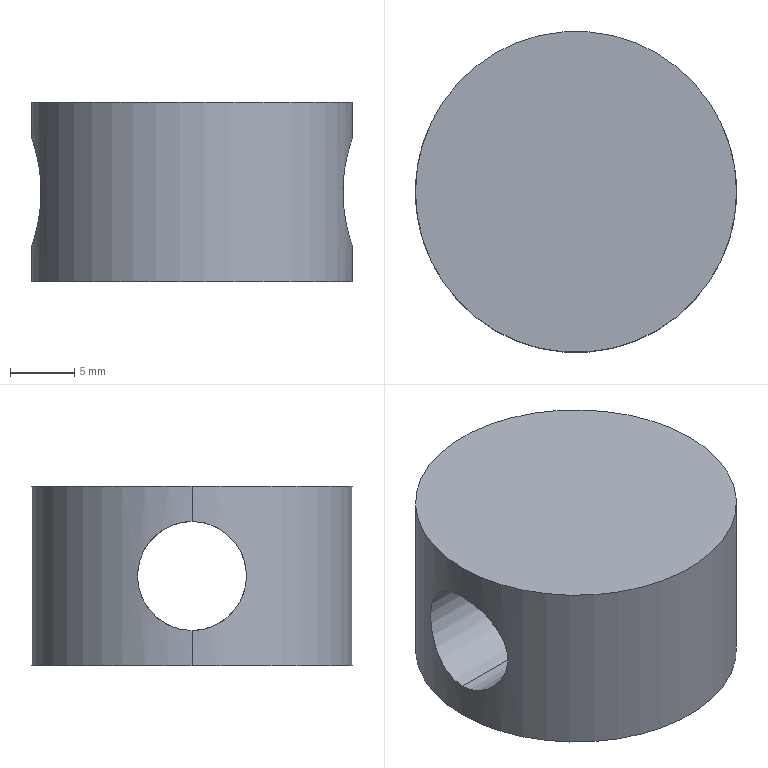Part | STEP file | Bronze shaft QY-1-15 | 1 solid | 6 faces | box 25 x 25 x 14 mm | volume 5474 mm3 | cylinder 4 | plane 2 | commonest cylinder face diameters 8.5 x2 25 x2
STEP:
#1=CARTESIAN_POINT('',(0.,0.,0.));
#2=DIRECTION('',(0.,0.,1.));
#3=DIRECTION('',(1.,0.,0.));
#4=AXIS2_PLACEMENT_3D('',#1,#2,#3);
#5=CARTESIAN_POINT('',(12.5,0.,11.25));
#6=VERTEX_POINT('',#5);
#7=CARTESIAN_POINT('',(-12.5,0.,11.25));
#8=VERTEX_POINT('',#7);
#9=CARTESIAN_POINT('',(0.,0.,11.25));
#10=DIRECTION('',(-1.,0.,0.));
#11=VECTOR('',#10,1.);
#12=LINE('',#9,#11);
#13=CARTESIAN_POINT('',(0.,0.,7.));
#14=DIRECTION('',(-1.,0.,0.));
#15=DIRECTION('',(0.,0.,1.));
#16=AXIS2_PLACEMENT_3D('',#13,#14,#15);
#17=CYLINDRICAL_SURFACE('',#16,4.25);
#18=CARTESIAN_POINT('',(6.283,0.));
#19=DIRECTION('',(0.,1.));
#20=VECTOR('',#19,1.);
#21=LINE('',#18,#20);
#22=(GEOMETRIC_REPRESENTATION_CONTEXT(2)PARAMETRIC_REPRESENTATION_CONTEXT()REPRESENTATION_CONTEXT('',''));
#23=DEFINITIONAL_REPRESENTATION('',(#21),#22);
#24=PCURVE('',#17,#23);
#25=CARTESIAN_POINT('',(0.,0.,7.));
#26=DIRECTION('',(-1.,0.,0.));
#27=DIRECTION('',(0.,0.,1.));
#28=AXIS2_PLACEMENT_3D('',#25,#26,#27);
#29=CYLINDRICAL_SURFACE('',#28,4.25);
#30=CARTESIAN_POINT('',(0.,0.));
#31=DIRECTION('',(0.,1.));
#32=VECTOR('',#31,1.);
#33=LINE('',#30,#32);
#34=(GEOMETRIC_REPRESENTATION_CONTEXT(2)PARAMETRIC_REPRESENTATION_CONTEXT()REPRESENTATION_CONTEXT('',''));
#35=DEFINITIONAL_REPRESENTATION('',(#33),#34);
#36=PCURVE('',#29,#35);
#37=SURFACE_CURVE('',#12,(#24,#36),.PCURVE_S1.);
#38=EDGE_CURVE('',#6,#8,#37,.T.);
#39=ORIENTED_EDGE('',*,*,#38,.T.);
#40=CARTESIAN_POINT('',(-12.5,0.,2.75));
#41=VERTEX_POINT('',#40);
#42=CARTESIAN_POINT('',(-12.5,0.,11.25));
#43=CARTESIAN_POINT('',(-12.5,-0.2831,11.25));
#44=CARTESIAN_POINT('',(-12.49,-0.561,11.222));
#45=CARTESIAN_POINT('',(-12.454,-1.107,11.113));
#46=CARTESIAN_POINT('',(-12.426,-1.378,11.03));
#47=CARTESIAN_POINT('',(-12.359,-1.892,10.816));
#48=CARTESIAN_POINT('',(-12.318,-2.136,10.685));
#49=CARTESIAN_POINT('',(-12.23,-2.596,10.376));
#50=CARTESIAN_POINT('',(-12.181,-2.812,10.198));
#51=CARTESIAN_POINT('',(-12.085,-3.201,9.809));
#52=CARTESIAN_POINT('',(-12.037,-3.376,9.597));
#53=CARTESIAN_POINT('',(-11.945,-3.687,9.133));
#54=CARTESIAN_POINT('',(-11.903,-3.817,8.889));
#55=CARTESIAN_POINT('',(-11.833,-4.03,8.379));
#56=CARTESIAN_POINT('',(-11.804,-4.112,8.109));
#57=CARTESIAN_POINT('',(-11.765,-4.222,7.559));
#58=CARTESIAN_POINT('',(-11.755,-4.25,7.282));
#59=CARTESIAN_POINT('',(-11.755,-4.25,6.723));
#60=CARTESIAN_POINT('',(-11.766,-4.222,6.439));
#61=CARTESIAN_POINT('',(-11.804,-4.112,5.892));
#62=CARTESIAN_POINT('',(-11.833,-4.031,5.626));
#63=CARTESIAN_POINT('',(-11.904,-3.816,5.108));
#64=CARTESIAN_POINT('',(-11.946,-3.684,4.864));
#65=CARTESIAN_POINT('',(-12.036,-3.377,4.405));
#66=CARTESIAN_POINT('',(-12.085,-3.2,4.189));
#67=CARTESIAN_POINT('',(-12.182,-2.808,3.798));
#68=CARTESIAN_POINT('',(-12.23,-2.596,3.624));
#69=CARTESIAN_POINT('',(-12.318,-2.137,3.316));
#70=CARTESIAN_POINT('',(-12.359,-1.888,3.182));
#71=CARTESIAN_POINT('',(-12.427,-1.376,2.97));
#72=CARTESIAN_POINT('',(-12.454,-1.111,2.888));
#73=CARTESIAN_POINT('',(-12.49,-0.5605,2.778));
#74=CARTESIAN_POINT('',(-12.5,-0.2789,2.75));
#75=CARTESIAN_POINT('',(-12.5,0.,2.75));
#76=B_SPLINE_CURVE_WITH_KNOTS('',3,(#42,#43,#44,#45,#46,#47,#48,#49,#50,#51,#52,#53,#54,#55,#56,#57,#58,#59,#60,#61,#62,#63,#64,#65,#66,#67,#68,#69,#70,#71,#72,#73,#74,#75),.UNSPECIFIED.,.F.,.F.,(4,2,2,2,2,2,2,2,2,2,2,2,2,2,2,2,4),(0.,0.0008368,0.001674,0.00251,0.003347,0.004184,0.005021,0.005857,0.006694,0.007531,0.008368,0.009204,0.01004,0.01088,0.01171,0.01255,0.01339),.UNSPECIFIED.);
#77=CARTESIAN_POINT('',(6.283,12.5));
#78=CARTESIAN_POINT('',(6.267,12.5));
#79=CARTESIAN_POINT('',(6.235,12.499));
#80=CARTESIAN_POINT('',(6.187,12.494));
#81=CARTESIAN_POINT('',(6.139,12.486));
#82=CARTESIAN_POINT('',(6.092,12.474));
#83=CARTESIAN_POINT('',(6.044,12.46));
#84=CARTESIAN_POINT('',(5.996,12.442));
#85=CARTESIAN_POINT('',(5.948,12.422));
#86=CARTESIAN_POINT('',(5.9,12.399));
#87=CARTESIAN_POINT('',(5.853,12.374));
#88=CARTESIAN_POINT('',(5.805,12.346));
#89=CARTESIAN_POINT('',(5.758,12.317));
#90=CARTESIAN_POINT('',(5.711,12.286));
#91=CARTESIAN_POINT('',(5.663,12.254));
#92=CARTESIAN_POINT('',(5.616,12.22));
#93=CARTESIAN_POINT('',(5.568,12.186));
#94=CARTESIAN_POINT('',(5.521,12.151));
#95=CARTESIAN_POINT('',(5.474,12.116));
#96=CARTESIAN_POINT('',(5.427,12.081));
#97=CARTESIAN_POINT('',(5.38,12.046));
#98=CARTESIAN_POINT('',(5.332,12.012));
#99=CARTESIAN_POINT('',(5.284,11.978));
#100=CARTESIAN_POINT('',(5.237,11.946));
#101=CARTESIAN_POINT('',(5.19,11.916));
#102=CARTESIAN_POINT('',(5.142,11.888));
#103=CARTESIAN_POINT('',(5.095,11.862));
#104=CARTESIAN_POINT('',(5.048,11.838));
#105=CARTESIAN_POINT('',(5.,11.816));
#106=CARTESIAN_POINT('',(4.952,11.798));
#107=CARTESIAN_POINT('',(4.904,11.783));
#108=CARTESIAN_POINT('',(4.856,11.77));
#109=CARTESIAN_POINT('',(4.808,11.762));
#110=CARTESIAN_POINT('',(4.761,11.757));
#111=CARTESIAN_POINT('',(4.713,11.755));
#112=CARTESIAN_POINT('',(4.665,11.756));
#113=CARTESIAN_POINT('',(4.617,11.762));
#114=CARTESIAN_POINT('',(4.569,11.771));
#115=CARTESIAN_POINT('',(4.521,11.783));
#116=CARTESIAN_POINT('',(4.473,11.798));
#117=CARTESIAN_POINT('',(4.425,11.816));
#118=CARTESIAN_POINT('',(4.378,11.837));
#119=CARTESIAN_POINT('',(4.33,11.861));
#120=CARTESIAN_POINT('',(4.282,11.888));
#121=CARTESIAN_POINT('',(4.234,11.916));
#122=CARTESIAN_POINT('',(4.187,11.947));
#123=CARTESIAN_POINT('',(4.14,11.979));
#124=CARTESIAN_POINT('',(4.093,12.012));
#125=CARTESIAN_POINT('',(4.045,12.046));
#126=CARTESIAN_POINT('',(3.998,12.081));
#127=CARTESIAN_POINT('',(3.95,12.116));
#128=CARTESIAN_POINT('',(3.903,12.151));
#129=CARTESIAN_POINT('',(3.856,12.186));
#130=CARTESIAN_POINT('',(3.809,12.22));
#131=CARTESIAN_POINT('',(3.762,12.254));
#132=CARTESIAN_POINT('',(3.714,12.286));
#133=CARTESIAN_POINT('',(3.667,12.317));
#134=CARTESIAN_POINT('',(3.619,12.347));
#135=CARTESIAN_POINT('',(3.571,12.374));
#136=CARTESIAN_POINT('',(3.524,12.399));
#137=CARTESIAN_POINT('',(3.477,12.422));
#138=CARTESIAN_POINT('',(3.429,12.442));
#139=CARTESIAN_POINT('',(3.382,12.46));
#140=CARTESIAN_POINT('',(3.334,12.474));
#141=CARTESIAN_POINT('',(3.285,12.486));
#142=CARTESIAN_POINT('',(3.237,12.494));
#143=CARTESIAN_POINT('',(3.189,12.499));
#144=CARTESIAN_POINT('',(3.157,12.5));
#145=CARTESIAN_POINT('',(3.142,12.5));
#146=B_SPLINE_CURVE_WITH_KNOTS('',3,(#77,#78,#79,#80,#81,#82,#83,#84,#85,#86,#87,#88,#89,#90,#91,#92,#93,#94,#95,#96,#97,#98,#99,#100,#101,#102,#103,#104,#105,#106,#107,#108,#109,#110,#111,#112,#113,#114,#115,#116,#117,#118,#119,#120,#121,#122,#123,#124,#125,#126,#127,#128,#129,#130,#131,#132,#133,#134,#135,#136,#137,#138,#139,#140,#141,#142,#143,#144,#145),.UNSPECIFIED.,.F.,.F.,(4,1,1,1,1,1,1,1,1,1,1,1,1,1,1,1,1,1,1,1,1,1,1,1,1,1,1,1,1,1,1,1,1,1,1,1,1,1,1,1,1,1,1,1,1,1,1,1,1,1,1,1,1,1,1,1,1,1,1,1,1,1,1,1,1,1,4),(0.,0.0002028,0.0004057,0.0006085,0.0008114,0.001014,0.001217,0.00142,0.001623,0.001826,0.002028,0.002231,0.002434,0.002637,0.00284,0.003043,0.003246,0.003448,0.003651,0.003854,0.004057,0.00426,0.004463,0.004666,0.004868,0.005071,0.005274,0.005477,0.00568,0.005883,0.006085,0.006288,0.006491,0.006694,0.006897,0.0071,0.007303,0.007505,0.007708,0.007911,0.008114,0.008317,0.00852,0.008722,0.008925,0.009128,0.009331,0.009534,0.009737,0.00994,0.01014,0.01035,0.01055,0.01075,0.01095,0.01116,0.01136,0.01156,0.01177,0.01197,0.01217,0.01237,0.01258,0.01278,0.01298,0.01319,0.01339),.QUASI_UNIFORM_KNOTS.);
#147=(GEOMETRIC_REPRESENTATION_CONTEXT(2)PARAMETRIC_REPRESENTATION_CONTEXT()REPRESENTATION_CONTEXT('',''));
#148=DEFINITIONAL_REPRESENTATION('',(#146),#147);
#149=PCURVE('',#17,#148);
#150=CARTESIAN_POINT('',(0.,0.,14.));
#151=DIRECTION('',(0.,0.,-1.));
#152=DIRECTION('',(-1.,0.,0.));
#153=AXIS2_PLACEMENT_3D('',#150,#151,#152);
#154=CYLINDRICAL_SURFACE('',#153,12.5);
#155=CARTESIAN_POINT('',(6.283,2.75));
#156=CARTESIAN_POINT('',(6.278,2.75));
#157=CARTESIAN_POINT('',(6.267,2.753));
#158=CARTESIAN_POINT('',(6.251,2.768));
#159=CARTESIAN_POINT('',(6.234,2.792));
#160=CARTESIAN_POINT('',(6.218,2.826));
#161=CARTESIAN_POINT('',(6.202,2.87));
#162=CARTESIAN_POINT('',(6.187,2.923));
#163=CARTESIAN_POINT('',(6.171,2.985));
#164=CARTESIAN_POINT('',(6.156,3.057));
#165=CARTESIAN_POINT('',(6.141,3.137));
#166=CARTESIAN_POINT('',(6.126,3.225));
#167=CARTESIAN_POINT('',(6.112,3.322));
#168=CARTESIAN_POINT('',(6.098,3.426));
#169=CARTESIAN_POINT('',(6.084,3.54));
#170=CARTESIAN_POINT('',(6.071,3.661));
#171=CARTESIAN_POINT('',(6.058,3.79));
#172=CARTESIAN_POINT('',(6.046,3.925));
#173=CARTESIAN_POINT('',(6.034,4.067));
#174=CARTESIAN_POINT('',(6.023,4.215));
#175=CARTESIAN_POINT('',(6.013,4.369));
#176=CARTESIAN_POINT('',(6.003,4.53));
#177=CARTESIAN_POINT('',(5.993,4.698));
#178=CARTESIAN_POINT('',(5.984,4.87));
#179=CARTESIAN_POINT('',(5.976,5.047));
#180=CARTESIAN_POINT('',(5.969,5.227));
#181=CARTESIAN_POINT('',(5.962,5.412));
#182=CARTESIAN_POINT('',(5.956,5.601));
#183=CARTESIAN_POINT('',(5.951,5.795));
#184=CARTESIAN_POINT('',(5.946,5.992));
#185=CARTESIAN_POINT('',(5.943,6.191));
#186=CARTESIAN_POINT('',(5.94,6.392));
#187=CARTESIAN_POINT('',(5.938,6.593));
#188=CARTESIAN_POINT('',(5.937,6.795));
#189=CARTESIAN_POINT('',(5.936,6.998));
#190=CARTESIAN_POINT('',(5.937,7.202));
#191=CARTESIAN_POINT('',(5.938,7.406));
#192=CARTESIAN_POINT('',(5.94,7.61));
#193=CARTESIAN_POINT('',(5.943,7.811));
#194=CARTESIAN_POINT('',(5.946,8.008));
#195=CARTESIAN_POINT('',(5.951,8.204));
#196=CARTESIAN_POINT('',(5.956,8.396));
#197=CARTESIAN_POINT('',(5.962,8.586));
#198=CARTESIAN_POINT('',(5.969,8.774));
#199=CARTESIAN_POINT('',(5.976,8.955));
#200=CARTESIAN_POINT('',(5.985,9.132));
#201=CARTESIAN_POINT('',(5.993,9.304));
#202=CARTESIAN_POINT('',(6.003,9.47));
#203=CARTESIAN_POINT('',(6.013,9.631));
#204=CARTESIAN_POINT('',(6.023,9.786));
#205=CARTESIAN_POINT('',(6.035,9.936));
#206=CARTESIAN_POINT('',(6.046,10.078));
#207=CARTESIAN_POINT('',(6.059,10.212));
#208=CARTESIAN_POINT('',(6.071,10.34));
#209=CARTESIAN_POINT('',(6.084,10.46));
#210=CARTESIAN_POINT('',(6.098,10.573));
#211=CARTESIAN_POINT('',(6.112,10.678));
#212=CARTESIAN_POINT('',(6.126,10.776));
#213=CARTESIAN_POINT('',(6.141,10.865));
#214=CARTESIAN_POINT('',(6.156,10.945));
#215=CARTESIAN_POINT('',(6.171,11.015));
#216=CARTESIAN_POINT('',(6.187,11.077));
#217=CARTESIAN_POINT('',(6.202,11.13));
#218=CARTESIAN_POINT('',(6.218,11.174));
#219=CARTESIAN_POINT('',(6.234,11.208));
#220=CARTESIAN_POINT('',(6.251,11.232));
#221=CARTESIAN_POINT('',(6.267,11.247));
#222=CARTESIAN_POINT('',(6.278,11.25));
#223=CARTESIAN_POINT('',(6.283,11.25));
#224=B_SPLINE_CURVE_WITH_KNOTS('',3,(#155,#156,#157,#158,#159,#160,#161,#162,#163,#164,#165,#166,#167,#168,#169,#170,#171,#172,#173,#174,#175,#176,#177,#178,#179,#180,#181,#182,#183,#184,#185,#186,#187,#188,#189,#190,#191,#192,#193,#194,#195,#196,#197,#198,#199,#200,#201,#202,#203,#204,#205,#206,#207,#208,#209,#210,#211,#212,#213,#214,#215,#216,#217,#218,#219,#220,#221,#222,#223),.UNSPECIFIED.,.F.,.F.,(4,1,1,1,1,1,1,1,1,1,1,1,1,1,1,1,1,1,1,1,1,1,1,1,1,1,1,1,1,1,1,1,1,1,1,1,1,1,1,1,1,1,1,1,1,1,1,1,1,1,1,1,1,1,1,1,1,1,1,1,1,1,1,1,1,1,4),(0.,0.0002028,0.0004057,0.0006085,0.0008114,0.001014,0.001217,0.00142,0.001623,0.001826,0.002028,0.002231,0.002434,0.002637,0.00284,0.003043,0.003246,0.003448,0.003651,0.003854,0.004057,0.00426,0.004463,0.004666,0.004868,0.005071,0.005274,0.005477,0.00568,0.005883,0.006085,0.006288,0.006491,0.006694,0.006897,0.0071,0.007303,0.007505,0.007708,0.007911,0.008114,0.008317,0.00852,0.008722,0.008925,0.009128,0.009331,0.009534,0.009737,0.00994,0.01014,0.01035,0.01055,0.01075,0.01095,0.01116,0.01136,0.01156,0.01177,0.01197,0.01217,0.01237,0.01258,0.01278,0.01298,0.01319,0.01339),.QUASI_UNIFORM_KNOTS.);
#225=(GEOMETRIC_REPRESENTATION_CONTEXT(2)PARAMETRIC_REPRESENTATION_CONTEXT()REPRESENTATION_CONTEXT('',''));
#226=DEFINITIONAL_REPRESENTATION('',(#224),#225);
#227=PCURVE('',#154,#226);
#228=SURFACE_CURVE('',#76,(#149,#227),.PCURVE_S1.);
#229=EDGE_CURVE('',#8,#41,#228,.T.);
#230=ORIENTED_EDGE('',*,*,#229,.T.);
#231=CARTESIAN_POINT('',(12.5,0.,2.75));
#232=VERTEX_POINT('',#231);
#233=CARTESIAN_POINT('',(0.,0.,2.75));
#234=DIRECTION('',(-1.,0.,0.));
#235=VECTOR('',#234,1.);
#236=LINE('',#233,#235);
#237=CARTESIAN_POINT('',(3.142,0.));
#238=DIRECTION('',(0.,1.));
#239=VECTOR('',#238,1.);
#240=LINE('',#237,#239);
#241=(GEOMETRIC_REPRESENTATION_CONTEXT(2)PARAMETRIC_REPRESENTATION_CONTEXT()REPRESENTATION_CONTEXT('',''));
#242=DEFINITIONAL_REPRESENTATION('',(#240),#241);
#243=PCURVE('',#17,#242);
#244=CARTESIAN_POINT('',(3.142,0.));
#245=DIRECTION('',(0.,1.));
#246=VECTOR('',#245,1.);
#247=LINE('',#244,#246);
#248=(GEOMETRIC_REPRESENTATION_CONTEXT(2)PARAMETRIC_REPRESENTATION_CONTEXT()REPRESENTATION_CONTEXT('',''));
#249=DEFINITIONAL_REPRESENTATION('',(#247),#248);
#250=PCURVE('',#29,#249);
#251=SURFACE_CURVE('',#236,(#243,#250),.PCURVE_S1.);
#252=EDGE_CURVE('',#232,#41,#251,.T.);
#253=ORIENTED_EDGE('',*,*,#252,.F.);
#254=CARTESIAN_POINT('',(12.5,0.,2.75));
#255=CARTESIAN_POINT('',(12.5,-0.2788,2.75));
#256=CARTESIAN_POINT('',(12.491,-0.5597,2.778));
#257=CARTESIAN_POINT('',(12.454,-1.111,2.888));
#258=CARTESIAN_POINT('',(12.427,-1.377,2.97));
#259=CARTESIAN_POINT('',(12.359,-1.89,3.183));
#260=CARTESIAN_POINT('',(12.318,-2.138,3.317));
#261=CARTESIAN_POINT('',(12.229,-2.597,3.624));
#262=CARTESIAN_POINT('',(12.182,-2.81,3.799));
#263=CARTESIAN_POINT('',(12.036,-3.398,4.388));
#264=CARTESIAN_POINT('',(11.939,-3.709,4.852));
#265=CARTESIAN_POINT('',(11.833,-4.031,5.626));
#266=CARTESIAN_POINT('',(11.804,-4.112,5.891));
#267=CARTESIAN_POINT('',(11.766,-4.222,6.437));
#268=CARTESIAN_POINT('',(11.755,-4.25,6.721));
#269=CARTESIAN_POINT('',(11.755,-4.25,7.281));
#270=CARTESIAN_POINT('',(11.765,-4.222,7.558));
#271=CARTESIAN_POINT('',(11.804,-4.113,8.108));
#272=CARTESIAN_POINT('',(11.833,-4.03,8.378));
#273=CARTESIAN_POINT('',(11.904,-3.817,8.89));
#274=CARTESIAN_POINT('',(11.946,-3.685,9.136));
#275=CARTESIAN_POINT('',(12.037,-3.375,9.598));
#276=CARTESIAN_POINT('',(12.085,-3.2,9.81));
#277=CARTESIAN_POINT('',(12.182,-2.811,10.2));
#278=CARTESIAN_POINT('',(12.23,-2.594,10.378));
#279=CARTESIAN_POINT('',(12.319,-2.135,10.685));
#280=CARTESIAN_POINT('',(12.359,-1.892,10.816));
#281=CARTESIAN_POINT('',(12.427,-1.378,11.03));
#282=CARTESIAN_POINT('',(12.454,-1.107,11.113));
#283=CARTESIAN_POINT('',(12.49,-0.561,11.222));
#284=CARTESIAN_POINT('',(12.5,-0.283,11.25));
#285=CARTESIAN_POINT('',(12.5,0.,11.25));
#286=B_SPLINE_CURVE_WITH_KNOTS('',3,(#254,#255,#256,#257,#258,#259,#260,#261,#262,#263,#264,#265,#266,#267,#268,#269,#270,#271,#272,#273,#274,#275,#276,#277,#278,#279,#280,#281,#282,#283,#284,#285),.UNSPECIFIED.,.F.,.F.,(4,2,2,2,2,2,2,2,2,2,2,2,2,2,2,4),(0.01339,0.01422,0.01506,0.0159,0.01673,0.01841,0.01924,0.02008,0.02092,0.02175,0.02259,0.02343,0.02426,0.0251,0.02594,0.02677),.UNSPECIFIED.);
#287=CARTESIAN_POINT('',(3.142,-12.5));
#288=CARTESIAN_POINT('',(3.157,-12.5));
#289=CARTESIAN_POINT('',(3.189,-12.499));
#290=CARTESIAN_POINT('',(3.237,-12.494));
#291=CARTESIAN_POINT('',(3.285,-12.486));
#292=CARTESIAN_POINT('',(3.333,-12.474));
#293=CARTESIAN_POINT('',(3.381,-12.46));
#294=CARTESIAN_POINT('',(3.429,-12.442));
#295=CARTESIAN_POINT('',(3.477,-12.422));
#296=CARTESIAN_POINT('',(3.524,-12.399));
#297=CARTESIAN_POINT('',(3.572,-12.374));
#298=CARTESIAN_POINT('',(3.619,-12.347));
#299=CARTESIAN_POINT('',(3.667,-12.317));
#300=CARTESIAN_POINT('',(3.715,-12.286));
#301=CARTESIAN_POINT('',(3.762,-12.254));
#302=CARTESIAN_POINT('',(3.809,-12.22));
#303=CARTESIAN_POINT('',(3.856,-12.186));
#304=CARTESIAN_POINT('',(3.903,-12.151));
#305=CARTESIAN_POINT('',(3.951,-12.115));
#306=CARTESIAN_POINT('',(3.998,-12.08));
#307=CARTESIAN_POINT('',(4.046,-12.045));
#308=CARTESIAN_POINT('',(4.093,-12.011));
#309=CARTESIAN_POINT('',(4.14,-11.978));
#310=CARTESIAN_POINT('',(4.187,-11.947));
#311=CARTESIAN_POINT('',(4.235,-11.916));
#312=CARTESIAN_POINT('',(4.282,-11.888));
#313=CARTESIAN_POINT('',(4.33,-11.861));
#314=CARTESIAN_POINT('',(4.378,-11.837));
#315=CARTESIAN_POINT('',(4.425,-11.816));
#316=CARTESIAN_POINT('',(4.473,-11.798));
#317=CARTESIAN_POINT('',(4.52,-11.783));
#318=CARTESIAN_POINT('',(4.568,-11.771));
#319=CARTESIAN_POINT('',(4.616,-11.762));
#320=CARTESIAN_POINT('',(4.665,-11.757));
#321=CARTESIAN_POINT('',(4.713,-11.755));
#322=CARTESIAN_POINT('',(4.76,-11.757));
#323=CARTESIAN_POINT('',(4.808,-11.762));
#324=CARTESIAN_POINT('',(4.856,-11.77));
#325=CARTESIAN_POINT('',(4.904,-11.782));
#326=CARTESIAN_POINT('',(4.952,-11.798));
#327=CARTESIAN_POINT('',(5.,-11.816));
#328=CARTESIAN_POINT('',(5.047,-11.838));
#329=CARTESIAN_POINT('',(5.095,-11.862));
#330=CARTESIAN_POINT('',(5.143,-11.888));
#331=CARTESIAN_POINT('',(5.19,-11.916));
#332=CARTESIAN_POINT('',(5.238,-11.947));
#333=CARTESIAN_POINT('',(5.285,-11.979));
#334=CARTESIAN_POINT('',(5.333,-12.012));
#335=CARTESIAN_POINT('',(5.38,-12.046));
#336=CARTESIAN_POINT('',(5.427,-12.081));
#337=CARTESIAN_POINT('',(5.474,-12.116));
#338=CARTESIAN_POINT('',(5.521,-12.151));
#339=CARTESIAN_POINT('',(5.569,-12.186));
#340=CARTESIAN_POINT('',(5.616,-12.221));
#341=CARTESIAN_POINT('',(5.664,-12.254));
#342=CARTESIAN_POINT('',(5.711,-12.287));
#343=CARTESIAN_POINT('',(5.758,-12.317));
#344=CARTESIAN_POINT('',(5.805,-12.347));
#345=CARTESIAN_POINT('',(5.853,-12.374));
#346=CARTESIAN_POINT('',(5.9,-12.399));
#347=CARTESIAN_POINT('',(5.948,-12.422));
#348=CARTESIAN_POINT('',(5.996,-12.442));
#349=CARTESIAN_POINT('',(6.044,-12.46));
#350=CARTESIAN_POINT('',(6.092,-12.474));
#351=CARTESIAN_POINT('',(6.139,-12.486));
#352=CARTESIAN_POINT('',(6.187,-12.494));
#353=CARTESIAN_POINT('',(6.235,-12.499));
#354=CARTESIAN_POINT('',(6.267,-12.5));
#355=CARTESIAN_POINT('',(6.283,-12.5));
#356=B_SPLINE_CURVE_WITH_KNOTS('',3,(#287,#288,#289,#290,#291,#292,#293,#294,#295,#296,#297,#298,#299,#300,#301,#302,#303,#304,#305,#306,#307,#308,#309,#310,#311,#312,#313,#314,#315,#316,#317,#318,#319,#320,#321,#322,#323,#324,#325,#326,#327,#328,#329,#330,#331,#332,#333,#334,#335,#336,#337,#338,#339,#340,#341,#342,#343,#344,#345,#346,#347,#348,#349,#350,#351,#352,#353,#354,#355),.UNSPECIFIED.,.F.,.F.,(4,1,1,1,1,1,1,1,1,1,1,1,1,1,1,1,1,1,1,1,1,1,1,1,1,1,1,1,1,1,1,1,1,1,1,1,1,1,1,1,1,1,1,1,1,1,1,1,1,1,1,1,1,1,1,1,1,1,1,1,1,1,1,1,1,1,4),(0.01339,0.01359,0.01379,0.014,0.0142,0.0144,0.0146,0.01481,0.01501,0.01521,0.01542,0.01562,0.01582,0.01602,0.01623,0.01643,0.01663,0.01684,0.01704,0.01724,0.01744,0.01765,0.01785,0.01805,0.01826,0.01846,0.01866,0.01886,0.01907,0.01927,0.01947,0.01967,0.01988,0.02008,0.02028,0.02049,0.02069,0.02089,0.02109,0.0213,0.0215,0.0217,0.02191,0.02211,0.02231,0.02251,0.02272,0.02292,0.02312,0.02333,0.02353,0.02373,0.02393,0.02414,0.02434,0.02454,0.02474,0.02495,0.02515,0.02535,0.02556,0.02576,0.02596,0.02616,0.02637,0.02657,0.02677),.QUASI_UNIFORM_KNOTS.);
#357=(GEOMETRIC_REPRESENTATION_CONTEXT(2)PARAMETRIC_REPRESENTATION_CONTEXT()REPRESENTATION_CONTEXT('',''));
#358=DEFINITIONAL_REPRESENTATION('',(#356),#357);
#359=PCURVE('',#17,#358);
#360=CARTESIAN_POINT('',(3.142,11.25));
#361=CARTESIAN_POINT('',(3.147,11.25));
#362=CARTESIAN_POINT('',(3.158,11.247));
#363=CARTESIAN_POINT('',(3.174,11.232));
#364=CARTESIAN_POINT('',(3.19,11.208));
#365=CARTESIAN_POINT('',(3.206,11.174));
#366=CARTESIAN_POINT('',(3.222,11.13));
#367=CARTESIAN_POINT('',(3.238,11.077));
#368=CARTESIAN_POINT('',(3.254,11.015));
#369=CARTESIAN_POINT('',(3.269,10.944));
#370=CARTESIAN_POINT('',(3.284,10.864));
#371=CARTESIAN_POINT('',(3.299,10.775));
#372=CARTESIAN_POINT('',(3.313,10.678));
#373=CARTESIAN_POINT('',(3.327,10.572));
#374=CARTESIAN_POINT('',(3.341,10.459));
#375=CARTESIAN_POINT('',(3.354,10.339));
#376=CARTESIAN_POINT('',(3.366,10.211));
#377=CARTESIAN_POINT('',(3.379,10.076));
#378=CARTESIAN_POINT('',(3.39,9.933));
#379=CARTESIAN_POINT('',(3.402,9.784));
#380=CARTESIAN_POINT('',(3.412,9.629));
#381=CARTESIAN_POINT('',(3.422,9.469));
#382=CARTESIAN_POINT('',(3.432,9.303));
#383=CARTESIAN_POINT('',(3.44,9.131));
#384=CARTESIAN_POINT('',(3.448,8.954));
#385=CARTESIAN_POINT('',(3.456,8.773));
#386=CARTESIAN_POINT('',(3.463,8.586));
#387=CARTESIAN_POINT('',(3.469,8.396));
#388=CARTESIAN_POINT('',(3.474,8.204));
#389=CARTESIAN_POINT('',(3.478,8.009));
#390=CARTESIAN_POINT('',(3.482,7.812));
#391=CARTESIAN_POINT('',(3.485,7.611));
#392=CARTESIAN_POINT('',(3.487,7.408));
#393=CARTESIAN_POINT('',(3.488,7.203));
#394=CARTESIAN_POINT('',(3.489,6.999));
#395=CARTESIAN_POINT('',(3.488,6.796));
#396=CARTESIAN_POINT('',(3.487,6.594));
#397=CARTESIAN_POINT('',(3.485,6.392));
#398=CARTESIAN_POINT('',(3.482,6.192));
#399=CARTESIAN_POINT('',(3.478,5.993));
#400=CARTESIAN_POINT('',(3.474,5.796));
#401=CARTESIAN_POINT('',(3.469,5.602));
#402=CARTESIAN_POINT('',(3.463,5.412));
#403=CARTESIAN_POINT('',(3.456,5.227));
#404=CARTESIAN_POINT('',(3.448,5.046));
#405=CARTESIAN_POINT('',(3.44,4.868));
#406=CARTESIAN_POINT('',(3.431,4.696));
#407=CARTESIAN_POINT('',(3.422,4.529));
#408=CARTESIAN_POINT('',(3.412,4.368));
#409=CARTESIAN_POINT('',(3.401,4.214));
#410=CARTESIAN_POINT('',(3.39,4.066));
#411=CARTESIAN_POINT('',(3.379,3.924));
#412=CARTESIAN_POINT('',(3.366,3.788));
#413=CARTESIAN_POINT('',(3.354,3.66));
#414=CARTESIAN_POINT('',(3.34,3.538));
#415=CARTESIAN_POINT('',(3.327,3.426));
#416=CARTESIAN_POINT('',(3.313,3.321));
#417=CARTESIAN_POINT('',(3.299,3.225));
#418=CARTESIAN_POINT('',(3.284,3.136));
#419=CARTESIAN_POINT('',(3.269,3.056));
#420=CARTESIAN_POINT('',(3.254,2.985));
#421=CARTESIAN_POINT('',(3.238,2.923));
#422=CARTESIAN_POINT('',(3.222,2.869));
#423=CARTESIAN_POINT('',(3.206,2.826));
#424=CARTESIAN_POINT('',(3.19,2.792));
#425=CARTESIAN_POINT('',(3.174,2.768));
#426=CARTESIAN_POINT('',(3.158,2.753));
#427=CARTESIAN_POINT('',(3.147,2.75));
#428=CARTESIAN_POINT('',(3.142,2.75));
#429=B_SPLINE_CURVE_WITH_KNOTS('',3,(#360,#361,#362,#363,#364,#365,#366,#367,#368,#369,#370,#371,#372,#373,#374,#375,#376,#377,#378,#379,#380,#381,#382,#383,#384,#385,#386,#387,#388,#389,#390,#391,#392,#393,#394,#395,#396,#397,#398,#399,#400,#401,#402,#403,#404,#405,#406,#407,#408,#409,#410,#411,#412,#413,#414,#415,#416,#417,#418,#419,#420,#421,#422,#423,#424,#425,#426,#427,#428),.UNSPECIFIED.,.F.,.F.,(4,1,1,1,1,1,1,1,1,1,1,1,1,1,1,1,1,1,1,1,1,1,1,1,1,1,1,1,1,1,1,1,1,1,1,1,1,1,1,1,1,1,1,1,1,1,1,1,1,1,1,1,1,1,1,1,1,1,1,1,1,1,1,1,1,1,4),(0.01339,0.01359,0.01379,0.014,0.0142,0.0144,0.0146,0.01481,0.01501,0.01521,0.01542,0.01562,0.01582,0.01602,0.01623,0.01643,0.01663,0.01684,0.01704,0.01724,0.01744,0.01765,0.01785,0.01805,0.01826,0.01846,0.01866,0.01886,0.01907,0.01927,0.01947,0.01967,0.01988,0.02008,0.02028,0.02049,0.02069,0.02089,0.02109,0.0213,0.0215,0.0217,0.02191,0.02211,0.02231,0.02251,0.02272,0.02292,0.02312,0.02333,0.02353,0.02373,0.02393,0.02414,0.02434,0.02454,0.02474,0.02495,0.02515,0.02535,0.02556,0.02576,0.02596,0.02616,0.02637,0.02657,0.02677),.QUASI_UNIFORM_KNOTS.);
#430=(GEOMETRIC_REPRESENTATION_CONTEXT(2)PARAMETRIC_REPRESENTATION_CONTEXT()REPRESENTATION_CONTEXT('',''));
#431=DEFINITIONAL_REPRESENTATION('',(#429),#430);
#432=PCURVE('',#154,#431);
#433=SURFACE_CURVE('',#286,(#359,#432),.PCURVE_S1.);
#434=EDGE_CURVE('',#232,#6,#433,.T.);
#435=ORIENTED_EDGE('',*,*,#434,.T.);
#436=EDGE_LOOP('',(#39,#230,#253,#435));
#437=FACE_BOUND('',#436,.F.);
#438=ADVANCED_FACE('',(#437),#17,.F.);
#439=CARTESIAN_POINT('',(12.5,0.,14.));
#440=VERTEX_POINT('',#439);
#441=CARTESIAN_POINT('',(-12.5,0.,14.));
#442=VERTEX_POINT('',#441);
#443=CARTESIAN_POINT('',(0.,0.,14.));
#444=DIRECTION('',(0.,0.,1.));
#445=DIRECTION('',(1.,0.,0.));
#446=AXIS2_PLACEMENT_3D('',#443,#444,#445);
#447=CIRCLE('',#446,12.5);
#448=CARTESIAN_POINT('',(0.,0.,14.));
#449=DIRECTION('',(0.,0.,-1.));
#450=DIRECTION('',(-1.,0.,0.));
#451=AXIS2_PLACEMENT_3D('',#448,#449,#450);
#452=CYLINDRICAL_SURFACE('',#451,12.5);
#453=CARTESIAN_POINT('',(3.142,0.));
#454=DIRECTION('',(-1.,0.));
#455=VECTOR('',#454,1.);
#456=LINE('',#453,#455);
#457=(GEOMETRIC_REPRESENTATION_CONTEXT(2)PARAMETRIC_REPRESENTATION_CONTEXT()REPRESENTATION_CONTEXT('',''));
#458=DEFINITIONAL_REPRESENTATION('',(#456),#457);
#459=PCURVE('',#452,#458);
#460=CARTESIAN_POINT('',(0.,0.,14.));
#461=DIRECTION('',(0.,0.,1.));
#462=DIRECTION('',(1.,0.,0.));
#463=AXIS2_PLACEMENT_3D('',#460,#461,#462);
#464=PLANE('',#463);
#465=CARTESIAN_POINT('',(0.,0.));
#466=DIRECTION('',(1.,0.));
#467=AXIS2_PLACEMENT_2D('',#465,#466);
#468=CIRCLE('',#467,12.5);
#469=(GEOMETRIC_REPRESENTATION_CONTEXT(2)PARAMETRIC_REPRESENTATION_CONTEXT()REPRESENTATION_CONTEXT('',''));
#470=DEFINITIONAL_REPRESENTATION('',(#468),#469);
#471=PCURVE('',#464,#470);
#472=SURFACE_CURVE('',#447,(#459,#471),.PCURVE_S1.);
#473=EDGE_CURVE('',#440,#442,#472,.T.);
#474=ORIENTED_EDGE('',*,*,#473,.F.);
#475=CARTESIAN_POINT('',(12.5,0.,14.));
#476=DIRECTION('',(0.,0.,-1.));
#477=VECTOR('',#476,1.);
#478=LINE('',#475,#477);
#479=CARTESIAN_POINT('',(3.142,0.));
#480=DIRECTION('',(0.,1.));
#481=VECTOR('',#480,1.);
#482=LINE('',#479,#481);
#483=(GEOMETRIC_REPRESENTATION_CONTEXT(2)PARAMETRIC_REPRESENTATION_CONTEXT()REPRESENTATION_CONTEXT('',''));
#484=DEFINITIONAL_REPRESENTATION('',(#482),#483);
#485=PCURVE('',#452,#484);
#486=CARTESIAN_POINT('',(3.142,0.));
#487=DIRECTION('',(0.,1.));
#488=VECTOR('',#487,1.);
#489=LINE('',#486,#488);
#490=(GEOMETRIC_REPRESENTATION_CONTEXT(2)PARAMETRIC_REPRESENTATION_CONTEXT()REPRESENTATION_CONTEXT('',''));
#491=DEFINITIONAL_REPRESENTATION('',(#489),#490);
#492=PCURVE('',#154,#491);
#493=SURFACE_CURVE('',#478,(#485,#492),.PCURVE_S1.);
#494=EDGE_CURVE('',#440,#6,#493,.T.);
#495=ORIENTED_EDGE('',*,*,#494,.T.);
#496=CARTESIAN_POINT('',(12.5,0.,11.25));
#497=CARTESIAN_POINT('',(12.5,0.2831,11.25));
#498=CARTESIAN_POINT('',(12.49,0.561,11.222));
#499=CARTESIAN_POINT('',(12.454,1.107,11.113));
#500=CARTESIAN_POINT('',(12.426,1.378,11.03));
#501=CARTESIAN_POINT('',(12.359,1.892,10.816));
#502=CARTESIAN_POINT('',(12.318,2.136,10.685));
#503=CARTESIAN_POINT('',(12.23,2.596,10.376));
#504=CARTESIAN_POINT('',(12.181,2.812,10.198));
#505=CARTESIAN_POINT('',(12.085,3.201,9.809));
#506=CARTESIAN_POINT('',(12.037,3.376,9.597));
#507=CARTESIAN_POINT('',(11.945,3.687,9.133));
#508=CARTESIAN_POINT('',(11.903,3.817,8.889));
#509=CARTESIAN_POINT('',(11.833,4.03,8.379));
#510=CARTESIAN_POINT('',(11.804,4.112,8.109));
#511=CARTESIAN_POINT('',(11.765,4.222,7.559));
#512=CARTESIAN_POINT('',(11.755,4.25,7.282));
#513=CARTESIAN_POINT('',(11.755,4.25,6.723));
#514=CARTESIAN_POINT('',(11.766,4.222,6.439));
#515=CARTESIAN_POINT('',(11.804,4.112,5.892));
#516=CARTESIAN_POINT('',(11.833,4.031,5.626));
#517=CARTESIAN_POINT('',(11.904,3.816,5.108));
#518=CARTESIAN_POINT('',(11.946,3.684,4.864));
#519=CARTESIAN_POINT('',(12.036,3.377,4.405));
#520=CARTESIAN_POINT('',(12.085,3.2,4.189));
#521=CARTESIAN_POINT('',(12.182,2.808,3.798));
#522=CARTESIAN_POINT('',(12.23,2.596,3.624));
#523=CARTESIAN_POINT('',(12.318,2.137,3.316));
#524=CARTESIAN_POINT('',(12.359,1.888,3.182));
#525=CARTESIAN_POINT('',(12.427,1.376,2.97));
#526=CARTESIAN_POINT('',(12.454,1.111,2.888));
#527=CARTESIAN_POINT('',(12.49,0.5605,2.778));
#528=CARTESIAN_POINT('',(12.5,0.2789,2.75));
#529=CARTESIAN_POINT('',(12.5,0.,2.75));
#530=B_SPLINE_CURVE_WITH_KNOTS('',3,(#496,#497,#498,#499,#500,#501,#502,#503,#504,#505,#506,#507,#508,#509,#510,#511,#512,#513,#514,#515,#516,#517,#518,#519,#520,#521,#522,#523,#524,#525,#526,#527,#528,#529),.UNSPECIFIED.,.F.,.F.,(4,2,2,2,2,2,2,2,2,2,2,2,2,2,2,2,4),(0.,0.0008368,0.001674,0.00251,0.003347,0.004184,0.005021,0.005857,0.006694,0.007531,0.008368,0.009204,0.01004,0.01088,0.01171,0.01255,0.01339),.UNSPECIFIED.);
#531=CARTESIAN_POINT('',(3.142,2.75));
#532=CARTESIAN_POINT('',(3.136,2.75));
#533=CARTESIAN_POINT('',(3.125,2.753));
#534=CARTESIAN_POINT('',(3.109,2.768));
#535=CARTESIAN_POINT('',(3.093,2.792));
#536=CARTESIAN_POINT('',(3.077,2.826));
#537=CARTESIAN_POINT('',(3.061,2.87));
#538=CARTESIAN_POINT('',(3.045,2.923));
#539=CARTESIAN_POINT('',(3.029,2.985));
#540=CARTESIAN_POINT('',(3.014,3.057));
#541=CARTESIAN_POINT('',(2.999,3.137));
#542=CARTESIAN_POINT('',(2.984,3.225));
#543=CARTESIAN_POINT('',(2.97,3.322));
#544=CARTESIAN_POINT('',(2.956,3.426));
#545=CARTESIAN_POINT('',(2.943,3.54));
#546=CARTESIAN_POINT('',(2.929,3.661));
#547=CARTESIAN_POINT('',(2.917,3.79));
#548=CARTESIAN_POINT('',(2.904,3.925));
#549=CARTESIAN_POINT('',(2.893,4.067));
#550=CARTESIAN_POINT('',(2.882,4.215));
#551=CARTESIAN_POINT('',(2.871,4.369));
#552=CARTESIAN_POINT('',(2.861,4.53));
#553=CARTESIAN_POINT('',(2.852,4.698));
#554=CARTESIAN_POINT('',(2.843,4.87));
#555=CARTESIAN_POINT('',(2.835,5.047));
#556=CARTESIAN_POINT('',(2.827,5.227));
#557=CARTESIAN_POINT('',(2.821,5.412));
#558=CARTESIAN_POINT('',(2.815,5.601));
#559=CARTESIAN_POINT('',(2.809,5.795));
#560=CARTESIAN_POINT('',(2.805,5.992));
#561=CARTESIAN_POINT('',(2.801,6.191));
#562=CARTESIAN_POINT('',(2.798,6.392));
#563=CARTESIAN_POINT('',(2.796,6.593));
#564=CARTESIAN_POINT('',(2.795,6.795));
#565=CARTESIAN_POINT('',(2.795,6.998));
#566=CARTESIAN_POINT('',(2.795,7.202));
#567=CARTESIAN_POINT('',(2.796,7.406));
#568=CARTESIAN_POINT('',(2.798,7.61));
#569=CARTESIAN_POINT('',(2.801,7.811));
#570=CARTESIAN_POINT('',(2.805,8.008));
#571=CARTESIAN_POINT('',(2.809,8.204));
#572=CARTESIAN_POINT('',(2.815,8.396));
#573=CARTESIAN_POINT('',(2.821,8.586));
#574=CARTESIAN_POINT('',(2.827,8.774));
#575=CARTESIAN_POINT('',(2.835,8.955));
#576=CARTESIAN_POINT('',(2.843,9.132));
#577=CARTESIAN_POINT('',(2.852,9.304));
#578=CARTESIAN_POINT('',(2.861,9.47));
#579=CARTESIAN_POINT('',(2.871,9.631));
#580=CARTESIAN_POINT('',(2.882,9.786));
#581=CARTESIAN_POINT('',(2.893,9.936));
#582=CARTESIAN_POINT('',(2.905,10.078));
#583=CARTESIAN_POINT('',(2.917,10.212));
#584=CARTESIAN_POINT('',(2.93,10.34));
#585=CARTESIAN_POINT('',(2.943,10.46));
#586=CARTESIAN_POINT('',(2.956,10.573));
#587=CARTESIAN_POINT('',(2.97,10.678));
#588=CARTESIAN_POINT('',(2.985,10.776));
#589=CARTESIAN_POINT('',(2.999,10.865));
#590=CARTESIAN_POINT('',(3.014,10.945));
#591=CARTESIAN_POINT('',(3.03,11.015));
#592=CARTESIAN_POINT('',(3.045,11.077));
#593=CARTESIAN_POINT('',(3.061,11.13));
#594=CARTESIAN_POINT('',(3.077,11.174));
#595=CARTESIAN_POINT('',(3.093,11.208));
#596=CARTESIAN_POINT('',(3.109,11.232));
#597=CARTESIAN_POINT('',(3.125,11.247));
#598=CARTESIAN_POINT('',(3.136,11.25));
#599=CARTESIAN_POINT('',(3.142,11.25));
#600=B_SPLINE_CURVE_WITH_KNOTS('',3,(#531,#532,#533,#534,#535,#536,#537,#538,#539,#540,#541,#542,#543,#544,#545,#546,#547,#548,#549,#550,#551,#552,#553,#554,#555,#556,#557,#558,#559,#560,#561,#562,#563,#564,#565,#566,#567,#568,#569,#570,#571,#572,#573,#574,#575,#576,#577,#578,#579,#580,#581,#582,#583,#584,#585,#586,#587,#588,#589,#590,#591,#592,#593,#594,#595,#596,#597,#598,#599),.UNSPECIFIED.,.F.,.F.,(4,1,1,1,1,1,1,1,1,1,1,1,1,1,1,1,1,1,1,1,1,1,1,1,1,1,1,1,1,1,1,1,1,1,1,1,1,1,1,1,1,1,1,1,1,1,1,1,1,1,1,1,1,1,1,1,1,1,1,1,1,1,1,1,1,1,4),(0.,0.0002028,0.0004057,0.0006085,0.0008114,0.001014,0.001217,0.00142,0.001623,0.001826,0.002028,0.002231,0.002434,0.002637,0.00284,0.003043,0.003246,0.003448,0.003651,0.003854,0.004057,0.00426,0.004463,0.004666,0.004868,0.005071,0.005274,0.005477,0.00568,0.005883,0.006085,0.006288,0.006491,0.006694,0.006897,0.0071,0.007303,0.007505,0.007708,0.007911,0.008114,0.008317,0.00852,0.008722,0.008925,0.009128,0.009331,0.009534,0.009737,0.00994,0.01014,0.01035,0.01055,0.01075,0.01095,0.01116,0.01136,0.01156,0.01177,0.01197,0.01217,0.01237,0.01258,0.01278,0.01298,0.01319,0.01339),.QUASI_UNIFORM_KNOTS.);
#601=(GEOMETRIC_REPRESENTATION_CONTEXT(2)PARAMETRIC_REPRESENTATION_CONTEXT()REPRESENTATION_CONTEXT('',''));
#602=DEFINITIONAL_REPRESENTATION('',(#600),#601);
#603=PCURVE('',#452,#602);
#604=CARTESIAN_POINT('',(0.,-12.5));
#605=CARTESIAN_POINT('',(0.01615,-12.5));
#606=CARTESIAN_POINT('',(0.0483,-12.499));
#607=CARTESIAN_POINT('',(0.09622,-12.494));
#608=CARTESIAN_POINT('',(0.1439,-12.486));
#609=CARTESIAN_POINT('',(0.1916,-12.474));
#610=CARTESIAN_POINT('',(0.2393,-12.46));
#611=CARTESIAN_POINT('',(0.2873,-12.442));
#612=CARTESIAN_POINT('',(0.3352,-12.422));
#613=CARTESIAN_POINT('',(0.3831,-12.399));
#614=CARTESIAN_POINT('',(0.4306,-12.374));
#615=CARTESIAN_POINT('',(0.478,-12.346));
#616=CARTESIAN_POINT('',(0.5253,-12.317));
#617=CARTESIAN_POINT('',(0.5726,-12.286));
#618=CARTESIAN_POINT('',(0.62,-12.254));
#619=CARTESIAN_POINT('',(0.6675,-12.22));
#620=CARTESIAN_POINT('',(0.715,-12.186));
#621=CARTESIAN_POINT('',(0.7623,-12.151));
#622=CARTESIAN_POINT('',(0.8094,-12.116));
#623=CARTESIAN_POINT('',(0.8564,-12.081));
#624=CARTESIAN_POINT('',(0.9036,-12.046));
#625=CARTESIAN_POINT('',(0.9509,-12.012));
#626=CARTESIAN_POINT('',(0.9987,-11.978));
#627=CARTESIAN_POINT('',(1.046,-11.946));
#628=CARTESIAN_POINT('',(1.094,-11.916));
#629=CARTESIAN_POINT('',(1.141,-11.888));
#630=CARTESIAN_POINT('',(1.188,-11.862));
#631=CARTESIAN_POINT('',(1.236,-11.838));
#632=CARTESIAN_POINT('',(1.283,-11.816));
#633=CARTESIAN_POINT('',(1.331,-11.798));
#634=CARTESIAN_POINT('',(1.379,-11.783));
#635=CARTESIAN_POINT('',(1.427,-11.77));
#636=CARTESIAN_POINT('',(1.475,-11.762));
#637=CARTESIAN_POINT('',(1.523,-11.757));
#638=CARTESIAN_POINT('',(1.57,-11.755));
#639=CARTESIAN_POINT('',(1.618,-11.756));
#640=CARTESIAN_POINT('',(1.666,-11.762));
#641=CARTESIAN_POINT('',(1.715,-11.771));
#642=CARTESIAN_POINT('',(1.763,-11.783));
#643=CARTESIAN_POINT('',(1.81,-11.798));
#644=CARTESIAN_POINT('',(1.858,-11.816));
#645=CARTESIAN_POINT('',(1.905,-11.837));
#646=CARTESIAN_POINT('',(1.953,-11.861));
#647=CARTESIAN_POINT('',(2.001,-11.888));
#648=CARTESIAN_POINT('',(2.049,-11.916));
#649=CARTESIAN_POINT('',(2.096,-11.947));
#650=CARTESIAN_POINT('',(2.143,-11.979));
#651=CARTESIAN_POINT('',(2.191,-12.012));
#652=CARTESIAN_POINT('',(2.238,-12.046));
#653=CARTESIAN_POINT('',(2.285,-12.081));
#654=CARTESIAN_POINT('',(2.333,-12.116));
#655=CARTESIAN_POINT('',(2.38,-12.151));
#656=CARTESIAN_POINT('',(2.427,-12.186));
#657=CARTESIAN_POINT('',(2.474,-12.22));
#658=CARTESIAN_POINT('',(2.521,-12.254));
#659=CARTESIAN_POINT('',(2.569,-12.286));
#660=CARTESIAN_POINT('',(2.616,-12.317));
#661=CARTESIAN_POINT('',(2.664,-12.347));
#662=CARTESIAN_POINT('',(2.712,-12.374));
#663=CARTESIAN_POINT('',(2.759,-12.399));
#664=CARTESIAN_POINT('',(2.807,-12.422));
#665=CARTESIAN_POINT('',(2.854,-12.442));
#666=CARTESIAN_POINT('',(2.902,-12.46));
#667=CARTESIAN_POINT('',(2.95,-12.474));
#668=CARTESIAN_POINT('',(2.998,-12.486));
#669=CARTESIAN_POINT('',(3.046,-12.494));
#670=CARTESIAN_POINT('',(3.094,-12.499));
#671=CARTESIAN_POINT('',(3.126,-12.5));
#672=CARTESIAN_POINT('',(3.142,-12.5));
#673=B_SPLINE_CURVE_WITH_KNOTS('',3,(#604,#605,#606,#607,#608,#609,#610,#611,#612,#613,#614,#615,#616,#617,#618,#619,#620,#621,#622,#623,#624,#625,#626,#627,#628,#629,#630,#631,#632,#633,#634,#635,#636,#637,#638,#639,#640,#641,#642,#643,#644,#645,#646,#647,#648,#649,#650,#651,#652,#653,#654,#655,#656,#657,#658,#659,#660,#661,#662,#663,#664,#665,#666,#667,#668,#669,#670,#671,#672),.UNSPECIFIED.,.F.,.F.,(4,1,1,1,1,1,1,1,1,1,1,1,1,1,1,1,1,1,1,1,1,1,1,1,1,1,1,1,1,1,1,1,1,1,1,1,1,1,1,1,1,1,1,1,1,1,1,1,1,1,1,1,1,1,1,1,1,1,1,1,1,1,1,1,1,1,4),(0.,0.0002028,0.0004057,0.0006085,0.0008114,0.001014,0.001217,0.00142,0.001623,0.001826,0.002028,0.002231,0.002434,0.002637,0.00284,0.003043,0.003246,0.003448,0.003651,0.003854,0.004057,0.00426,0.004463,0.004666,0.004868,0.005071,0.005274,0.005477,0.00568,0.005883,0.006085,0.006288,0.006491,0.006694,0.006897,0.0071,0.007303,0.007505,0.007708,0.007911,0.008114,0.008317,0.00852,0.008722,0.008925,0.009128,0.009331,0.009534,0.009737,0.00994,0.01014,0.01035,0.01055,0.01075,0.01095,0.01116,0.01136,0.01156,0.01177,0.01197,0.01217,0.01237,0.01258,0.01278,0.01298,0.01319,0.01339),.QUASI_UNIFORM_KNOTS.);
#674=(GEOMETRIC_REPRESENTATION_CONTEXT(2)PARAMETRIC_REPRESENTATION_CONTEXT()REPRESENTATION_CONTEXT('',''));
#675=DEFINITIONAL_REPRESENTATION('',(#673),#674);
#676=PCURVE('',#29,#675);
#677=SURFACE_CURVE('',#530,(#603,#676),.PCURVE_S1.);
#678=EDGE_CURVE('',#6,#232,#677,.T.);
#679=ORIENTED_EDGE('',*,*,#678,.T.);
#680=CARTESIAN_POINT('',(12.5,0.,0.));
#681=VERTEX_POINT('',#680);
#682=CARTESIAN_POINT('',(12.5,0.,14.));
#683=DIRECTION('',(0.,0.,-1.));
#684=VECTOR('',#683,1.);
#685=LINE('',#682,#684);
#686=CARTESIAN_POINT('',(3.142,0.));
#687=DIRECTION('',(0.,1.));
#688=VECTOR('',#687,1.);
#689=LINE('',#686,#688);
#690=(GEOMETRIC_REPRESENTATION_CONTEXT(2)PARAMETRIC_REPRESENTATION_CONTEXT()REPRESENTATION_CONTEXT('',''));
#691=DEFINITIONAL_REPRESENTATION('',(#689),#690);
#692=PCURVE('',#452,#691);
#693=CARTESIAN_POINT('',(3.142,0.));
#694=DIRECTION('',(0.,1.));
#695=VECTOR('',#694,1.);
#696=LINE('',#693,#695);
#697=(GEOMETRIC_REPRESENTATION_CONTEXT(2)PARAMETRIC_REPRESENTATION_CONTEXT()REPRESENTATION_CONTEXT('',''));
#698=DEFINITIONAL_REPRESENTATION('',(#696),#697);
#699=PCURVE('',#154,#698);
#700=SURFACE_CURVE('',#685,(#692,#699),.PCURVE_S1.);
#701=EDGE_CURVE('',#232,#681,#700,.T.);
#702=ORIENTED_EDGE('',*,*,#701,.T.);
#703=CARTESIAN_POINT('',(-12.5,0.,0.));
#704=VERTEX_POINT('',#703);
#705=CARTESIAN_POINT('',(0.,0.,0.));
#706=DIRECTION('',(0.,0.,1.));
#707=DIRECTION('',(1.,0.,0.));
#708=AXIS2_PLACEMENT_3D('',#705,#706,#707);
#709=CIRCLE('',#708,12.5);
#710=CARTESIAN_POINT('',(3.142,14.));
#711=DIRECTION('',(-1.,0.));
#712=VECTOR('',#711,1.);
#713=LINE('',#710,#712);
#714=(GEOMETRIC_REPRESENTATION_CONTEXT(2)PARAMETRIC_REPRESENTATION_CONTEXT()REPRESENTATION_CONTEXT('',''));
#715=DEFINITIONAL_REPRESENTATION('',(#713),#714);
#716=PCURVE('',#452,#715);
#717=CARTESIAN_POINT('',(0.,0.,0.));
#718=DIRECTION('',(0.,0.,1.));
#719=DIRECTION('',(1.,0.,0.));
#720=AXIS2_PLACEMENT_3D('',#717,#718,#719);
#721=PLANE('',#720);
#722=CARTESIAN_POINT('',(0.,0.));
#723=DIRECTION('',(1.,0.));
#724=AXIS2_PLACEMENT_2D('',#722,#723);
#725=CIRCLE('',#724,12.5);
#726=(GEOMETRIC_REPRESENTATION_CONTEXT(2)PARAMETRIC_REPRESENTATION_CONTEXT()REPRESENTATION_CONTEXT('',''));
#727=DEFINITIONAL_REPRESENTATION('',(#725),#726);
#728=PCURVE('',#721,#727);
#729=SURFACE_CURVE('',#709,(#716,#728),.PCURVE_S1.);
#730=EDGE_CURVE('',#681,#704,#729,.T.);
#731=ORIENTED_EDGE('',*,*,#730,.T.);
#732=CARTESIAN_POINT('',(-12.5,0.,14.));
#733=DIRECTION('',(0.,0.,-1.));
#734=VECTOR('',#733,1.);
#735=LINE('',#732,#734);
#736=CARTESIAN_POINT('',(0.,0.));
#737=DIRECTION('',(0.,1.));
#738=VECTOR('',#737,1.);
#739=LINE('',#736,#738);
#740=(GEOMETRIC_REPRESENTATION_CONTEXT(2)PARAMETRIC_REPRESENTATION_CONTEXT()REPRESENTATION_CONTEXT('',''));
#741=DEFINITIONAL_REPRESENTATION('',(#739),#740);
#742=PCURVE('',#452,#741);
#743=CARTESIAN_POINT('',(6.283,0.));
#744=DIRECTION('',(0.,1.));
#745=VECTOR('',#744,1.);
#746=LINE('',#743,#745);
#747=(GEOMETRIC_REPRESENTATION_CONTEXT(2)PARAMETRIC_REPRESENTATION_CONTEXT()REPRESENTATION_CONTEXT('',''));
#748=DEFINITIONAL_REPRESENTATION('',(#746),#747);
#749=PCURVE('',#154,#748);
#750=SURFACE_CURVE('',#735,(#742,#749),.PCURVE_S1.);
#751=EDGE_CURVE('',#41,#704,#750,.T.);
#752=ORIENTED_EDGE('',*,*,#751,.F.);
#753=CARTESIAN_POINT('',(-12.5,0.,2.75));
#754=CARTESIAN_POINT('',(-12.5,0.2788,2.75));
#755=CARTESIAN_POINT('',(-12.491,0.5597,2.778));
#756=CARTESIAN_POINT('',(-12.454,1.111,2.888));
#757=CARTESIAN_POINT('',(-12.427,1.377,2.97));
#758=CARTESIAN_POINT('',(-12.359,1.89,3.183));
#759=CARTESIAN_POINT('',(-12.318,2.138,3.317));
#760=CARTESIAN_POINT('',(-12.229,2.597,3.624));
#761=CARTESIAN_POINT('',(-12.182,2.81,3.799));
#762=CARTESIAN_POINT('',(-12.036,3.398,4.388));
#763=CARTESIAN_POINT('',(-11.939,3.709,4.852));
#764=CARTESIAN_POINT('',(-11.833,4.031,5.626));
#765=CARTESIAN_POINT('',(-11.804,4.112,5.891));
#766=CARTESIAN_POINT('',(-11.766,4.222,6.437));
#767=CARTESIAN_POINT('',(-11.755,4.25,6.721));
#768=CARTESIAN_POINT('',(-11.755,4.25,7.281));
#769=CARTESIAN_POINT('',(-11.765,4.222,7.558));
#770=CARTESIAN_POINT('',(-11.804,4.113,8.108));
#771=CARTESIAN_POINT('',(-11.833,4.03,8.378));
#772=CARTESIAN_POINT('',(-11.904,3.817,8.89));
#773=CARTESIAN_POINT('',(-11.946,3.685,9.136));
#774=CARTESIAN_POINT('',(-12.037,3.375,9.598));
#775=CARTESIAN_POINT('',(-12.085,3.2,9.81));
#776=CARTESIAN_POINT('',(-12.182,2.811,10.2));
#777=CARTESIAN_POINT('',(-12.23,2.594,10.378));
#778=CARTESIAN_POINT('',(-12.319,2.135,10.685));
#779=CARTESIAN_POINT('',(-12.359,1.892,10.816));
#780=CARTESIAN_POINT('',(-12.427,1.378,11.03));
#781=CARTESIAN_POINT('',(-12.454,1.107,11.113));
#782=CARTESIAN_POINT('',(-12.49,0.561,11.222));
#783=CARTESIAN_POINT('',(-12.5,0.283,11.25));
#784=CARTESIAN_POINT('',(-12.5,0.,11.25));
#785=B_SPLINE_CURVE_WITH_KNOTS('',3,(#753,#754,#755,#756,#757,#758,#759,#760,#761,#762,#763,#764,#765,#766,#767,#768,#769,#770,#771,#772,#773,#774,#775,#776,#777,#778,#779,#780,#781,#782,#783,#784),.UNSPECIFIED.,.F.,.F.,(4,2,2,2,2,2,2,2,2,2,2,2,2,2,2,4),(0.01339,0.01422,0.01506,0.0159,0.01673,0.01841,0.01924,0.02008,0.02092,0.02175,0.02259,0.02343,0.02426,0.0251,0.02594,0.02677),.UNSPECIFIED.);
#786=CARTESIAN_POINT('',(0.,11.25));
#787=CARTESIAN_POINT('',(0.005407,11.25));
#788=CARTESIAN_POINT('',(0.01624,11.247));
#789=CARTESIAN_POINT('',(0.03251,11.232));
#790=CARTESIAN_POINT('',(0.04874,11.208));
#791=CARTESIAN_POINT('',(0.0649,11.174));
#792=CARTESIAN_POINT('',(0.08089,11.13));
#793=CARTESIAN_POINT('',(0.09661,11.077));
#794=CARTESIAN_POINT('',(0.1121,11.015));
#795=CARTESIAN_POINT('',(0.1273,10.944));
#796=CARTESIAN_POINT('',(0.1423,10.864));
#797=CARTESIAN_POINT('',(0.1571,10.775));
#798=CARTESIAN_POINT('',(0.1715,10.678));
#799=CARTESIAN_POINT('',(0.1855,10.572));
#800=CARTESIAN_POINT('',(0.199,10.459));
#801=CARTESIAN_POINT('',(0.2121,10.339));
#802=CARTESIAN_POINT('',(0.2248,10.211));
#803=CARTESIAN_POINT('',(0.237,10.076));
#804=CARTESIAN_POINT('',(0.2488,9.933));
#805=CARTESIAN_POINT('',(0.26,9.784));
#806=CARTESIAN_POINT('',(0.2706,9.629));
#807=CARTESIAN_POINT('',(0.2806,9.469));
#808=CARTESIAN_POINT('',(0.29,9.303));
#809=CARTESIAN_POINT('',(0.2988,9.131));
#810=CARTESIAN_POINT('',(0.3069,8.954));
#811=CARTESIAN_POINT('',(0.3143,8.773));
#812=CARTESIAN_POINT('',(0.3211,8.586));
#813=CARTESIAN_POINT('',(0.3271,8.396));
#814=CARTESIAN_POINT('',(0.3323,8.204));
#815=CARTESIAN_POINT('',(0.3367,8.009));
#816=CARTESIAN_POINT('',(0.3404,7.812));
#817=CARTESIAN_POINT('',(0.3433,7.611));
#818=CARTESIAN_POINT('',(0.3454,7.408));
#819=CARTESIAN_POINT('',(0.3466,7.203));
#820=CARTESIAN_POINT('',(0.3471,6.999));
#821=CARTESIAN_POINT('',(0.3466,6.796));
#822=CARTESIAN_POINT('',(0.3454,6.594));
#823=CARTESIAN_POINT('',(0.3433,6.392));
#824=CARTESIAN_POINT('',(0.3405,6.192));
#825=CARTESIAN_POINT('',(0.3368,5.993));
#826=CARTESIAN_POINT('',(0.3323,5.796));
#827=CARTESIAN_POINT('',(0.327,5.602));
#828=CARTESIAN_POINT('',(0.321,5.412));
#829=CARTESIAN_POINT('',(0.3143,5.227));
#830=CARTESIAN_POINT('',(0.3068,5.046));
#831=CARTESIAN_POINT('',(0.2987,4.868));
#832=CARTESIAN_POINT('',(0.2899,4.696));
#833=CARTESIAN_POINT('',(0.2804,4.529));
#834=CARTESIAN_POINT('',(0.2704,4.368));
#835=CARTESIAN_POINT('',(0.2598,4.214));
#836=CARTESIAN_POINT('',(0.2487,4.066));
#837=CARTESIAN_POINT('',(0.237,3.924));
#838=CARTESIAN_POINT('',(0.2247,3.788));
#839=CARTESIAN_POINT('',(0.212,3.66));
#840=CARTESIAN_POINT('',(0.1988,3.538));
#841=CARTESIAN_POINT('',(0.1852,3.426));
#842=CARTESIAN_POINT('',(0.1713,3.321));
#843=CARTESIAN_POINT('',(0.157,3.225));
#844=CARTESIAN_POINT('',(0.1424,3.136));
#845=CARTESIAN_POINT('',(0.1274,3.056));
#846=CARTESIAN_POINT('',(0.1121,2.985));
#847=CARTESIAN_POINT('',(0.09647,2.923));
#848=CARTESIAN_POINT('',(0.08067,2.869));
#849=CARTESIAN_POINT('',(0.06478,2.826));
#850=CARTESIAN_POINT('',(0.0488,2.792));
#851=CARTESIAN_POINT('',(0.03268,2.768));
#852=CARTESIAN_POINT('',(0.01642,2.753));
#853=CARTESIAN_POINT('',(0.005489,2.75));
#854=CARTESIAN_POINT('',(0.,2.75));
#855=B_SPLINE_CURVE_WITH_KNOTS('',3,(#786,#787,#788,#789,#790,#791,#792,#793,#794,#795,#796,#797,#798,#799,#800,#801,#802,#803,#804,#805,#806,#807,#808,#809,#810,#811,#812,#813,#814,#815,#816,#817,#818,#819,#820,#821,#822,#823,#824,#825,#826,#827,#828,#829,#830,#831,#832,#833,#834,#835,#836,#837,#838,#839,#840,#841,#842,#843,#844,#845,#846,#847,#848,#849,#850,#851,#852,#853,#854),.UNSPECIFIED.,.F.,.F.,(4,1,1,1,1,1,1,1,1,1,1,1,1,1,1,1,1,1,1,1,1,1,1,1,1,1,1,1,1,1,1,1,1,1,1,1,1,1,1,1,1,1,1,1,1,1,1,1,1,1,1,1,1,1,1,1,1,1,1,1,1,1,1,1,1,1,4),(0.01339,0.01359,0.01379,0.014,0.0142,0.0144,0.0146,0.01481,0.01501,0.01521,0.01542,0.01562,0.01582,0.01602,0.01623,0.01643,0.01663,0.01684,0.01704,0.01724,0.01744,0.01765,0.01785,0.01805,0.01826,0.01846,0.01866,0.01886,0.01907,0.01927,0.01947,0.01967,0.01988,0.02008,0.02028,0.02049,0.02069,0.02089,0.02109,0.0213,0.0215,0.0217,0.02191,0.02211,0.02231,0.02251,0.02272,0.02292,0.02312,0.02333,0.02353,0.02373,0.02393,0.02414,0.02434,0.02454,0.02474,0.02495,0.02515,0.02535,0.02556,0.02576,0.02596,0.02616,0.02637,0.02657,0.02677),.QUASI_UNIFORM_KNOTS.);
#856=(GEOMETRIC_REPRESENTATION_CONTEXT(2)PARAMETRIC_REPRESENTATION_CONTEXT()REPRESENTATION_CONTEXT('',''));
#857=DEFINITIONAL_REPRESENTATION('',(#855),#856);
#858=PCURVE('',#452,#857);
#859=CARTESIAN_POINT('',(3.142,12.5));
#860=CARTESIAN_POINT('',(3.126,12.5));
#861=CARTESIAN_POINT('',(3.094,12.499));
#862=CARTESIAN_POINT('',(3.046,12.494));
#863=CARTESIAN_POINT('',(2.998,12.486));
#864=CARTESIAN_POINT('',(2.95,12.474));
#865=CARTESIAN_POINT('',(2.902,12.46));
#866=CARTESIAN_POINT('',(2.854,12.442));
#867=CARTESIAN_POINT('',(2.807,12.422));
#868=CARTESIAN_POINT('',(2.759,12.399));
#869=CARTESIAN_POINT('',(2.711,12.374));
#870=CARTESIAN_POINT('',(2.664,12.347));
#871=CARTESIAN_POINT('',(2.616,12.317));
#872=CARTESIAN_POINT('',(2.568,12.286));
#873=CARTESIAN_POINT('',(2.521,12.254));
#874=CARTESIAN_POINT('',(2.474,12.22));
#875=CARTESIAN_POINT('',(2.427,12.186));
#876=CARTESIAN_POINT('',(2.38,12.151));
#877=CARTESIAN_POINT('',(2.332,12.115));
#878=CARTESIAN_POINT('',(2.285,12.08));
#879=CARTESIAN_POINT('',(2.238,12.045));
#880=CARTESIAN_POINT('',(2.19,12.011));
#881=CARTESIAN_POINT('',(2.143,11.978));
#882=CARTESIAN_POINT('',(2.096,11.947));
#883=CARTESIAN_POINT('',(2.048,11.916));
#884=CARTESIAN_POINT('',(2.001,11.888));
#885=CARTESIAN_POINT('',(1.953,11.861));
#886=CARTESIAN_POINT('',(1.905,11.837));
#887=CARTESIAN_POINT('',(1.858,11.816));
#888=CARTESIAN_POINT('',(1.81,11.798));
#889=CARTESIAN_POINT('',(1.763,11.783));
#890=CARTESIAN_POINT('',(1.715,11.771));
#891=CARTESIAN_POINT('',(1.667,11.762));
#892=CARTESIAN_POINT('',(1.619,11.757));
#893=CARTESIAN_POINT('',(1.571,11.755));
#894=CARTESIAN_POINT('',(1.523,11.757));
#895=CARTESIAN_POINT('',(1.475,11.762));
#896=CARTESIAN_POINT('',(1.427,11.77));
#897=CARTESIAN_POINT('',(1.38,11.782));
#898=CARTESIAN_POINT('',(1.332,11.798));
#899=CARTESIAN_POINT('',(1.284,11.816));
#900=CARTESIAN_POINT('',(1.236,11.838));
#901=CARTESIAN_POINT('',(1.188,11.862));
#902=CARTESIAN_POINT('',(1.141,11.888));
#903=CARTESIAN_POINT('',(1.093,11.916));
#904=CARTESIAN_POINT('',(1.046,11.947));
#905=CARTESIAN_POINT('',(0.998,11.979));
#906=CARTESIAN_POINT('',(0.9505,12.012));
#907=CARTESIAN_POINT('',(0.9032,12.046));
#908=CARTESIAN_POINT('',(0.8561,12.081));
#909=CARTESIAN_POINT('',(0.8091,12.116));
#910=CARTESIAN_POINT('',(0.762,12.151));
#911=CARTESIAN_POINT('',(0.7145,12.186));
#912=CARTESIAN_POINT('',(0.667,12.221));
#913=CARTESIAN_POINT('',(0.6195,12.254));
#914=CARTESIAN_POINT('',(0.5722,12.287));
#915=CARTESIAN_POINT('',(0.525,12.317));
#916=CARTESIAN_POINT('',(0.4778,12.347));
#917=CARTESIAN_POINT('',(0.4305,12.374));
#918=CARTESIAN_POINT('',(0.3829,12.399));
#919=CARTESIAN_POINT('',(0.3351,12.422));
#920=CARTESIAN_POINT('',(0.2871,12.442));
#921=CARTESIAN_POINT('',(0.2392,12.46));
#922=CARTESIAN_POINT('',(0.1915,12.474));
#923=CARTESIAN_POINT('',(0.1439,12.486));
#924=CARTESIAN_POINT('',(0.0962,12.494));
#925=CARTESIAN_POINT('',(0.04829,12.499));
#926=CARTESIAN_POINT('',(0.01614,12.5));
#927=CARTESIAN_POINT('',(0.,12.5));
#928=B_SPLINE_CURVE_WITH_KNOTS('',3,(#859,#860,#861,#862,#863,#864,#865,#866,#867,#868,#869,#870,#871,#872,#873,#874,#875,#876,#877,#878,#879,#880,#881,#882,#883,#884,#885,#886,#887,#888,#889,#890,#891,#892,#893,#894,#895,#896,#897,#898,#899,#900,#901,#902,#903,#904,#905,#906,#907,#908,#909,#910,#911,#912,#913,#914,#915,#916,#917,#918,#919,#920,#921,#922,#923,#924,#925,#926,#927),.UNSPECIFIED.,.F.,.F.,(4,1,1,1,1,1,1,1,1,1,1,1,1,1,1,1,1,1,1,1,1,1,1,1,1,1,1,1,1,1,1,1,1,1,1,1,1,1,1,1,1,1,1,1,1,1,1,1,1,1,1,1,1,1,1,1,1,1,1,1,1,1,1,1,1,1,4),(0.01339,0.01359,0.01379,0.014,0.0142,0.0144,0.0146,0.01481,0.01501,0.01521,0.01542,0.01562,0.01582,0.01602,0.01623,0.01643,0.01663,0.01684,0.01704,0.01724,0.01744,0.01765,0.01785,0.01805,0.01826,0.01846,0.01866,0.01886,0.01907,0.01927,0.01947,0.01967,0.01988,0.02008,0.02028,0.02049,0.02069,0.02089,0.02109,0.0213,0.0215,0.0217,0.02191,0.02211,0.02231,0.02251,0.02272,0.02292,0.02312,0.02333,0.02353,0.02373,0.02393,0.02414,0.02434,0.02454,0.02474,0.02495,0.02515,0.02535,0.02556,0.02576,0.02596,0.02616,0.02637,0.02657,0.02677),.QUASI_UNIFORM_KNOTS.);
#929=(GEOMETRIC_REPRESENTATION_CONTEXT(2)PARAMETRIC_REPRESENTATION_CONTEXT()REPRESENTATION_CONTEXT('',''));
#930=DEFINITIONAL_REPRESENTATION('',(#928),#929);
#931=PCURVE('',#29,#930);
#932=SURFACE_CURVE('',#785,(#858,#931),.PCURVE_S1.);
#933=EDGE_CURVE('',#41,#8,#932,.T.);
#934=ORIENTED_EDGE('',*,*,#933,.T.);
#935=CARTESIAN_POINT('',(-12.5,0.,14.));
#936=DIRECTION('',(0.,0.,-1.));
#937=VECTOR('',#936,1.);
#938=LINE('',#935,#937);
#939=CARTESIAN_POINT('',(0.,0.));
#940=DIRECTION('',(0.,1.));
#941=VECTOR('',#940,1.);
#942=LINE('',#939,#941);
#943=(GEOMETRIC_REPRESENTATION_CONTEXT(2)PARAMETRIC_REPRESENTATION_CONTEXT()REPRESENTATION_CONTEXT('',''));
#944=DEFINITIONAL_REPRESENTATION('',(#942),#943);
#945=PCURVE('',#452,#944);
#946=CARTESIAN_POINT('',(6.283,0.));
#947=DIRECTION('',(0.,1.));
#948=VECTOR('',#947,1.);
#949=LINE('',#946,#948);
#950=(GEOMETRIC_REPRESENTATION_CONTEXT(2)PARAMETRIC_REPRESENTATION_CONTEXT()REPRESENTATION_CONTEXT('',''));
#951=DEFINITIONAL_REPRESENTATION('',(#949),#950);
#952=PCURVE('',#154,#951);
#953=SURFACE_CURVE('',#938,(#945,#952),.PCURVE_S1.);
#954=EDGE_CURVE('',#442,#8,#953,.T.);
#955=ORIENTED_EDGE('',*,*,#954,.F.);
#956=EDGE_LOOP('',(#474,#495,#679,#702,#731,#752,#934,#955));
#957=FACE_BOUND('',#956,.T.);
#958=ADVANCED_FACE('',(#957),#452,.T.);
#959=ORIENTED_EDGE('',*,*,#494,.F.);
#960=CARTESIAN_POINT('',(0.,0.,14.));
#961=DIRECTION('',(0.,0.,1.));
#962=DIRECTION('',(1.,0.,0.));
#963=AXIS2_PLACEMENT_3D('',#960,#961,#962);
#964=CIRCLE('',#963,12.5);
#965=CARTESIAN_POINT('',(9.425,0.));
#966=DIRECTION('',(-1.,0.));
#967=VECTOR('',#966,1.);
#968=LINE('',#965,#967);
#969=(GEOMETRIC_REPRESENTATION_CONTEXT(2)PARAMETRIC_REPRESENTATION_CONTEXT()REPRESENTATION_CONTEXT('',''));
#970=DEFINITIONAL_REPRESENTATION('',(#968),#969);
#971=PCURVE('',#154,#970);
#972=CARTESIAN_POINT('',(0.,0.));
#973=DIRECTION('',(1.,0.));
#974=AXIS2_PLACEMENT_2D('',#972,#973);
#975=CIRCLE('',#974,12.5);
#976=(GEOMETRIC_REPRESENTATION_CONTEXT(2)PARAMETRIC_REPRESENTATION_CONTEXT()REPRESENTATION_CONTEXT('',''));
#977=DEFINITIONAL_REPRESENTATION('',(#975),#976);
#978=PCURVE('',#464,#977);
#979=SURFACE_CURVE('',#964,(#971,#978),.PCURVE_S1.);
#980=EDGE_CURVE('',#442,#440,#979,.T.);
#981=ORIENTED_EDGE('',*,*,#980,.F.);
#982=ORIENTED_EDGE('',*,*,#954,.T.);
#983=ORIENTED_EDGE('',*,*,#229,.T.);
#984=ORIENTED_EDGE('',*,*,#751,.T.);
#985=CARTESIAN_POINT('',(0.,0.,0.));
#986=DIRECTION('',(0.,0.,1.));
#987=DIRECTION('',(1.,0.,0.));
#988=AXIS2_PLACEMENT_3D('',#985,#986,#987);
#989=CIRCLE('',#988,12.5);
#990=CARTESIAN_POINT('',(9.425,14.));
#991=DIRECTION('',(-1.,0.));
#992=VECTOR('',#991,1.);
#993=LINE('',#990,#992);
#994=(GEOMETRIC_REPRESENTATION_CONTEXT(2)PARAMETRIC_REPRESENTATION_CONTEXT()REPRESENTATION_CONTEXT('',''));
#995=DEFINITIONAL_REPRESENTATION('',(#993),#994);
#996=PCURVE('',#154,#995);
#997=CARTESIAN_POINT('',(0.,0.));
#998=DIRECTION('',(1.,0.));
#999=AXIS2_PLACEMENT_2D('',#997,#998);
#1000=CIRCLE('',#999,12.5);
#1001=(GEOMETRIC_REPRESENTATION_CONTEXT(2)PARAMETRIC_REPRESENTATION_CONTEXT()REPRESENTATION_CONTEXT('',''));
#1002=DEFINITIONAL_REPRESENTATION('',(#1000),#1001);
#1003=PCURVE('',#721,#1002);
#1004=SURFACE_CURVE('',#989,(#996,#1003),.PCURVE_S1.);
#1005=EDGE_CURVE('',#704,#681,#1004,.T.);
#1006=ORIENTED_EDGE('',*,*,#1005,.T.);
#1007=ORIENTED_EDGE('',*,*,#701,.F.);
#1008=ORIENTED_EDGE('',*,*,#434,.T.);
#1009=EDGE_LOOP('',(#959,#981,#982,#983,#984,#1006,#1007,#1008));
#1010=FACE_BOUND('',#1009,.T.);
#1011=ADVANCED_FACE('',(#1010),#154,.T.);
#1012=ORIENTED_EDGE('',*,*,#980,.T.);
#1013=ORIENTED_EDGE('',*,*,#473,.T.);
#1014=EDGE_LOOP('',(#1012,#1013));
#1015=FACE_BOUND('',#1014,.T.);
#1016=ADVANCED_FACE('',(#1015),#464,.T.);
#1017=ORIENTED_EDGE('',*,*,#1005,.F.);
#1018=ORIENTED_EDGE('',*,*,#730,.F.);
#1019=EDGE_LOOP('',(#1017,#1018));
#1020=FACE_BOUND('',#1019,.T.);
#1021=ADVANCED_FACE('',(#1020),#721,.F.);
#1022=ORIENTED_EDGE('',*,*,#933,.T.);
#1023=ORIENTED_EDGE('',*,*,#38,.F.);
#1024=ORIENTED_EDGE('',*,*,#678,.T.);
#1025=ORIENTED_EDGE('',*,*,#252,.T.);
#1026=EDGE_LOOP('',(#1022,#1023,#1024,#1025));
#1027=FACE_BOUND('',#1026,.F.);
#1028=ADVANCED_FACE('',(#1027),#29,.F.);
#1029=CLOSED_SHELL('',(#438,#958,#1011,#1016,#1021,#1028));
#1030=MANIFOLD_SOLID_BREP('',#1029);
#1031=(LENGTH_UNIT()NAMED_UNIT(*)SI_UNIT(.MILLI.,.METRE.));
#1032=UNCERTAINTY_MEASURE_WITH_UNIT(LENGTH_MEASURE(0.0001),#1031,'','');
#1033=(NAMED_UNIT(*)PLANE_ANGLE_UNIT()SI_UNIT($,.RADIAN.));
#1034=(NAMED_UNIT(*)SI_UNIT($,.STERADIAN.)SOLID_ANGLE_UNIT());
#1035=(GEOMETRIC_REPRESENTATION_CONTEXT(3)GLOBAL_UNCERTAINTY_ASSIGNED_CONTEXT((#1032))GLOBAL_UNIT_ASSIGNED_CONTEXT((#1031,#1033,#1034))REPRESENTATION_CONTEXT('',''));
#1036=ADVANCED_BREP_SHAPE_REPRESENTATION('',(#4,#1030),#1035);